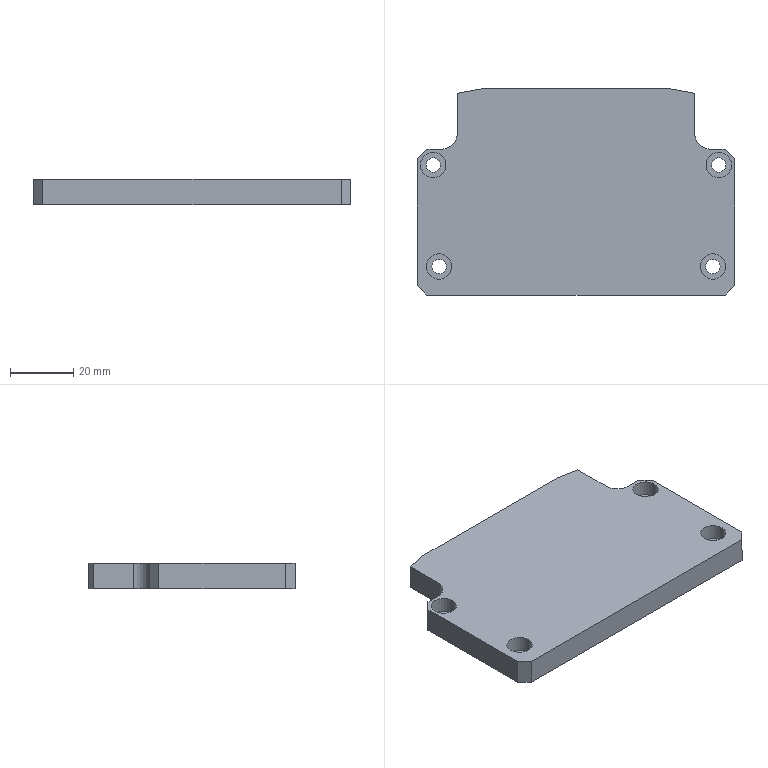Part | SolidWorks | features Chamfer 4, MoveFace 3, Fillet 2, HoleWzd 2, ICE 2, Extrusion 1 | 1 solid | 46 faces | box 100 x 65 x 8 mm | volume 46552 mm3 | cylinder 22 | plane 20 | cone 4 | commonest cylinder face diameters 4.5 x8 8 x8 3.3 x4 10 x2
STEP:
#1=CARTESIAN_POINT('',(-47.15,-14.,-1.));
#2=VERTEX_POINT('',#1);
#3=CARTESIAN_POINT('',(-39.15,-14.,-1.));
#4=VERTEX_POINT('',#3);
#5=CARTESIAN_POINT('',(-43.15,-14.,-1.));
#6=DIRECTION('',(0.,0.,1.));
#7=DIRECTION('',(1.,0.,0.));
#8=AXIS2_PLACEMENT_3D('',#5,#6,#7);
#9=CIRCLE('',#8,4.);
#10=EDGE_CURVE('',#2,#4,#9,.T.);
#11=ORIENTED_EDGE('',*,*,#10,.F.);
#12=CARTESIAN_POINT('',(-47.15,-14.,4.));
#13=VERTEX_POINT('',#12);
#14=CARTESIAN_POINT('',(-47.15,-14.,4.));
#15=DIRECTION('',(0.,0.,1.));
#16=VECTOR('',#15,1000.);
#17=LINE('',#14,#16);
#18=EDGE_CURVE('',#2,#13,#17,.T.);
#19=ORIENTED_EDGE('',*,*,#18,.T.);
#20=CARTESIAN_POINT('',(-39.15,-14.,4.));
#21=VERTEX_POINT('',#20);
#22=CARTESIAN_POINT('',(-43.15,-14.,4.));
#23=DIRECTION('',(0.,0.,1.));
#24=DIRECTION('',(1.,0.,0.));
#25=AXIS2_PLACEMENT_3D('',#22,#23,#24);
#26=CIRCLE('',#25,4.);
#27=EDGE_CURVE('',#13,#21,#26,.T.);
#28=ORIENTED_EDGE('',*,*,#27,.T.);
#29=CARTESIAN_POINT('',(-39.15,-14.,4.));
#30=DIRECTION('',(0.,0.,1.));
#31=VECTOR('',#30,1000.);
#32=LINE('',#29,#31);
#33=EDGE_CURVE('',#4,#21,#32,.T.);
#34=ORIENTED_EDGE('',*,*,#33,.F.);
#35=EDGE_LOOP('',(#11,#19,#28,#34));
#36=FACE_OUTER_BOUND('',#35,.T.);
#37=CARTESIAN_POINT('',(-43.15,-14.,4.));
#38=DIRECTION('',(0.,0.,1.));
#39=DIRECTION('',(1.,0.,0.));
#40=AXIS2_PLACEMENT_3D('',#37,#38,#39);
#41=CYLINDRICAL_SURFACE('',#40,4.);
#42=ADVANCED_FACE('',(#36),#41,.F.);
#43=CARTESIAN_POINT('',(-45.4,-14.,-4.));
#44=VERTEX_POINT('',#43);
#45=CARTESIAN_POINT('',(-40.9,-14.,-4.));
#46=VERTEX_POINT('',#45);
#47=CARTESIAN_POINT('',(-43.15,-14.,-4.));
#48=DIRECTION('',(0.,0.,1.));
#49=DIRECTION('',(1.,0.,0.));
#50=AXIS2_PLACEMENT_3D('',#47,#48,#49);
#51=CIRCLE('',#50,2.25);
#52=EDGE_CURVE('',#44,#46,#51,.T.);
#53=ORIENTED_EDGE('',*,*,#52,.F.);
#54=CARTESIAN_POINT('',(-45.4,-14.,-1.));
#55=VERTEX_POINT('',#54);
#56=CARTESIAN_POINT('',(-45.4,-14.,4.));
#57=DIRECTION('',(0.,0.,1.));
#58=VECTOR('',#57,1000.);
#59=LINE('',#56,#58);
#60=EDGE_CURVE('',#44,#55,#59,.T.);
#61=ORIENTED_EDGE('',*,*,#60,.T.);
#62=CARTESIAN_POINT('',(-40.9,-14.,-1.));
#63=VERTEX_POINT('',#62);
#64=CARTESIAN_POINT('',(-43.15,-14.,-1.));
#65=DIRECTION('',(0.,0.,1.));
#66=DIRECTION('',(1.,0.,0.));
#67=AXIS2_PLACEMENT_3D('',#64,#65,#66);
#68=CIRCLE('',#67,2.25);
#69=EDGE_CURVE('',#55,#63,#68,.T.);
#70=ORIENTED_EDGE('',*,*,#69,.T.);
#71=CARTESIAN_POINT('',(-40.9,-14.,4.));
#72=DIRECTION('',(0.,0.,1.));
#73=VECTOR('',#72,1000.);
#74=LINE('',#71,#73);
#75=EDGE_CURVE('',#46,#63,#74,.T.);
#76=ORIENTED_EDGE('',*,*,#75,.F.);
#77=EDGE_LOOP('',(#53,#61,#70,#76));
#78=FACE_OUTER_BOUND('',#77,.T.);
#79=CARTESIAN_POINT('',(-43.15,-14.,4.));
#80=DIRECTION('',(0.,0.,1.));
#81=DIRECTION('',(1.,0.,0.));
#82=AXIS2_PLACEMENT_3D('',#79,#80,#81);
#83=CYLINDRICAL_SURFACE('',#82,2.25);
#84=ADVANCED_FACE('',(#78),#83,.F.);
#85=CARTESIAN_POINT('',(39.15,-14.,-1.));
#86=VERTEX_POINT('',#85);
#87=CARTESIAN_POINT('',(47.15,-14.,-1.));
#88=VERTEX_POINT('',#87);
#89=CARTESIAN_POINT('',(43.15,-14.,-1.));
#90=DIRECTION('',(0.,0.,1.));
#91=DIRECTION('',(1.,0.,0.));
#92=AXIS2_PLACEMENT_3D('',#89,#90,#91);
#93=CIRCLE('',#92,4.);
#94=EDGE_CURVE('',#86,#88,#93,.T.);
#95=ORIENTED_EDGE('',*,*,#94,.F.);
#96=CARTESIAN_POINT('',(39.15,-14.,4.));
#97=VERTEX_POINT('',#96);
#98=CARTESIAN_POINT('',(39.15,-14.,4.));
#99=DIRECTION('',(0.,0.,1.));
#100=VECTOR('',#99,1000.);
#101=LINE('',#98,#100);
#102=EDGE_CURVE('',#86,#97,#101,.T.);
#103=ORIENTED_EDGE('',*,*,#102,.T.);
#104=CARTESIAN_POINT('',(47.15,-14.,4.));
#105=VERTEX_POINT('',#104);
#106=CARTESIAN_POINT('',(43.15,-14.,4.));
#107=DIRECTION('',(0.,0.,1.));
#108=DIRECTION('',(1.,0.,0.));
#109=AXIS2_PLACEMENT_3D('',#106,#107,#108);
#110=CIRCLE('',#109,4.);
#111=EDGE_CURVE('',#97,#105,#110,.T.);
#112=ORIENTED_EDGE('',*,*,#111,.T.);
#113=CARTESIAN_POINT('',(47.15,-14.,4.));
#114=DIRECTION('',(0.,0.,1.));
#115=VECTOR('',#114,1000.);
#116=LINE('',#113,#115);
#117=EDGE_CURVE('',#88,#105,#116,.T.);
#118=ORIENTED_EDGE('',*,*,#117,.F.);
#119=EDGE_LOOP('',(#95,#103,#112,#118));
#120=FACE_OUTER_BOUND('',#119,.T.);
#121=CARTESIAN_POINT('',(43.15,-14.,4.));
#122=DIRECTION('',(0.,0.,1.));
#123=DIRECTION('',(1.,0.,0.));
#124=AXIS2_PLACEMENT_3D('',#121,#122,#123);
#125=CYLINDRICAL_SURFACE('',#124,4.);
#126=ADVANCED_FACE('',(#120),#125,.F.);
#127=CARTESIAN_POINT('',(40.9,-14.,-4.));
#128=VERTEX_POINT('',#127);
#129=CARTESIAN_POINT('',(45.4,-14.,-4.));
#130=VERTEX_POINT('',#129);
#131=CARTESIAN_POINT('',(43.15,-14.,-4.));
#132=DIRECTION('',(0.,0.,1.));
#133=DIRECTION('',(1.,0.,0.));
#134=AXIS2_PLACEMENT_3D('',#131,#132,#133);
#135=CIRCLE('',#134,2.25);
#136=EDGE_CURVE('',#128,#130,#135,.T.);
#137=ORIENTED_EDGE('',*,*,#136,.F.);
#138=CARTESIAN_POINT('',(40.9,-14.,-1.));
#139=VERTEX_POINT('',#138);
#140=CARTESIAN_POINT('',(40.9,-14.,4.));
#141=DIRECTION('',(0.,0.,1.));
#142=VECTOR('',#141,1000.);
#143=LINE('',#140,#142);
#144=EDGE_CURVE('',#128,#139,#143,.T.);
#145=ORIENTED_EDGE('',*,*,#144,.T.);
#146=CARTESIAN_POINT('',(45.4,-14.,-1.));
#147=VERTEX_POINT('',#146);
#148=CARTESIAN_POINT('',(43.15,-14.,-1.));
#149=DIRECTION('',(0.,0.,1.));
#150=DIRECTION('',(1.,0.,0.));
#151=AXIS2_PLACEMENT_3D('',#148,#149,#150);
#152=CIRCLE('',#151,2.25);
#153=EDGE_CURVE('',#139,#147,#152,.T.);
#154=ORIENTED_EDGE('',*,*,#153,.T.);
#155=CARTESIAN_POINT('',(45.4,-14.,4.));
#156=DIRECTION('',(0.,0.,1.));
#157=VECTOR('',#156,1000.);
#158=LINE('',#155,#157);
#159=EDGE_CURVE('',#130,#147,#158,.T.);
#160=ORIENTED_EDGE('',*,*,#159,.F.);
#161=EDGE_LOOP('',(#137,#145,#154,#160));
#162=FACE_OUTER_BOUND('',#161,.T.);
#163=CARTESIAN_POINT('',(43.15,-14.,4.));
#164=DIRECTION('',(0.,0.,1.));
#165=DIRECTION('',(1.,0.,0.));
#166=AXIS2_PLACEMENT_3D('',#163,#164,#165);
#167=CYLINDRICAL_SURFACE('',#166,2.25);
#168=ADVANCED_FACE('',(#162),#167,.F.);
#169=CARTESIAN_POINT('',(-49.,18.,-1.));
#170=VERTEX_POINT('',#169);
#171=CARTESIAN_POINT('',(-41.,18.,-1.));
#172=VERTEX_POINT('',#171);
#173=CARTESIAN_POINT('',(-45.,18.,-1.));
#174=DIRECTION('',(0.,0.,1.));
#175=DIRECTION('',(1.,0.,0.));
#176=AXIS2_PLACEMENT_3D('',#173,#174,#175);
#177=CIRCLE('',#176,4.);
#178=EDGE_CURVE('',#170,#172,#177,.T.);
#179=ORIENTED_EDGE('',*,*,#178,.F.);
#180=CARTESIAN_POINT('',(-49.,18.,4.));
#181=VERTEX_POINT('',#180);
#182=CARTESIAN_POINT('',(-49.,18.,4.));
#183=DIRECTION('',(0.,0.,1.));
#184=VECTOR('',#183,1000.);
#185=LINE('',#182,#184);
#186=EDGE_CURVE('',#170,#181,#185,.T.);
#187=ORIENTED_EDGE('',*,*,#186,.T.);
#188=CARTESIAN_POINT('',(-41.,18.,4.));
#189=VERTEX_POINT('',#188);
#190=CARTESIAN_POINT('',(-45.,18.,4.));
#191=DIRECTION('',(0.,0.,1.));
#192=DIRECTION('',(1.,0.,0.));
#193=AXIS2_PLACEMENT_3D('',#190,#191,#192);
#194=CIRCLE('',#193,4.);
#195=EDGE_CURVE('',#181,#189,#194,.T.);
#196=ORIENTED_EDGE('',*,*,#195,.T.);
#197=CARTESIAN_POINT('',(-41.,18.,4.));
#198=DIRECTION('',(0.,0.,1.));
#199=VECTOR('',#198,1000.);
#200=LINE('',#197,#199);
#201=EDGE_CURVE('',#172,#189,#200,.T.);
#202=ORIENTED_EDGE('',*,*,#201,.F.);
#203=EDGE_LOOP('',(#179,#187,#196,#202));
#204=FACE_OUTER_BOUND('',#203,.T.);
#205=CARTESIAN_POINT('',(-45.,18.,4.));
#206=DIRECTION('',(0.,0.,1.));
#207=DIRECTION('',(1.,0.,0.));
#208=AXIS2_PLACEMENT_3D('',#205,#206,#207);
#209=CYLINDRICAL_SURFACE('',#208,4.);
#210=ADVANCED_FACE('',(#204),#209,.F.);
#211=CARTESIAN_POINT('',(-47.25,18.,-4.));
#212=VERTEX_POINT('',#211);
#213=CARTESIAN_POINT('',(-42.75,18.,-4.));
#214=VERTEX_POINT('',#213);
#215=CARTESIAN_POINT('',(-45.,18.,-4.));
#216=DIRECTION('',(0.,0.,1.));
#217=DIRECTION('',(1.,0.,0.));
#218=AXIS2_PLACEMENT_3D('',#215,#216,#217);
#219=CIRCLE('',#218,2.25);
#220=EDGE_CURVE('',#212,#214,#219,.T.);
#221=ORIENTED_EDGE('',*,*,#220,.F.);
#222=CARTESIAN_POINT('',(-47.25,18.,-1.));
#223=VERTEX_POINT('',#222);
#224=CARTESIAN_POINT('',(-47.25,18.,4.));
#225=DIRECTION('',(0.,0.,1.));
#226=VECTOR('',#225,1000.);
#227=LINE('',#224,#226);
#228=EDGE_CURVE('',#212,#223,#227,.T.);
#229=ORIENTED_EDGE('',*,*,#228,.T.);
#230=CARTESIAN_POINT('',(-42.75,18.,-1.));
#231=VERTEX_POINT('',#230);
#232=CARTESIAN_POINT('',(-45.,18.,-1.));
#233=DIRECTION('',(0.,0.,1.));
#234=DIRECTION('',(1.,0.,0.));
#235=AXIS2_PLACEMENT_3D('',#232,#233,#234);
#236=CIRCLE('',#235,2.25);
#237=EDGE_CURVE('',#223,#231,#236,.T.);
#238=ORIENTED_EDGE('',*,*,#237,.T.);
#239=CARTESIAN_POINT('',(-42.75,18.,4.));
#240=DIRECTION('',(0.,0.,1.));
#241=VECTOR('',#240,1000.);
#242=LINE('',#239,#241);
#243=EDGE_CURVE('',#214,#231,#242,.T.);
#244=ORIENTED_EDGE('',*,*,#243,.F.);
#245=EDGE_LOOP('',(#221,#229,#238,#244));
#246=FACE_OUTER_BOUND('',#245,.T.);
#247=CARTESIAN_POINT('',(-45.,18.,4.));
#248=DIRECTION('',(0.,0.,1.));
#249=DIRECTION('',(1.,0.,0.));
#250=AXIS2_PLACEMENT_3D('',#247,#248,#249);
#251=CYLINDRICAL_SURFACE('',#250,2.25);
#252=ADVANCED_FACE('',(#246),#251,.F.);
#253=CARTESIAN_POINT('',(41.,18.,-1.));
#254=VERTEX_POINT('',#253);
#255=CARTESIAN_POINT('',(49.,18.,-1.));
#256=VERTEX_POINT('',#255);
#257=CARTESIAN_POINT('',(45.,18.,-1.));
#258=DIRECTION('',(0.,0.,1.));
#259=DIRECTION('',(1.,0.,0.));
#260=AXIS2_PLACEMENT_3D('',#257,#258,#259);
#261=CIRCLE('',#260,4.);
#262=EDGE_CURVE('',#254,#256,#261,.T.);
#263=ORIENTED_EDGE('',*,*,#262,.F.);
#264=CARTESIAN_POINT('',(41.,18.,4.));
#265=VERTEX_POINT('',#264);
#266=CARTESIAN_POINT('',(41.,18.,4.));
#267=DIRECTION('',(0.,0.,1.));
#268=VECTOR('',#267,1000.);
#269=LINE('',#266,#268);
#270=EDGE_CURVE('',#254,#265,#269,.T.);
#271=ORIENTED_EDGE('',*,*,#270,.T.);
#272=CARTESIAN_POINT('',(49.,18.,4.));
#273=VERTEX_POINT('',#272);
#274=CARTESIAN_POINT('',(45.,18.,4.));
#275=DIRECTION('',(0.,0.,1.));
#276=DIRECTION('',(1.,0.,0.));
#277=AXIS2_PLACEMENT_3D('',#274,#275,#276);
#278=CIRCLE('',#277,4.);
#279=EDGE_CURVE('',#265,#273,#278,.T.);
#280=ORIENTED_EDGE('',*,*,#279,.T.);
#281=CARTESIAN_POINT('',(49.,18.,4.));
#282=DIRECTION('',(0.,0.,1.));
#283=VECTOR('',#282,1000.);
#284=LINE('',#281,#283);
#285=EDGE_CURVE('',#256,#273,#284,.T.);
#286=ORIENTED_EDGE('',*,*,#285,.F.);
#287=EDGE_LOOP('',(#263,#271,#280,#286));
#288=FACE_OUTER_BOUND('',#287,.T.);
#289=CARTESIAN_POINT('',(45.,18.,4.));
#290=DIRECTION('',(0.,0.,1.));
#291=DIRECTION('',(1.,0.,0.));
#292=AXIS2_PLACEMENT_3D('',#289,#290,#291);
#293=CYLINDRICAL_SURFACE('',#292,4.);
#294=ADVANCED_FACE('',(#288),#293,.F.);
#295=CARTESIAN_POINT('',(42.75,18.,-4.));
#296=VERTEX_POINT('',#295);
#297=CARTESIAN_POINT('',(47.25,18.,-4.));
#298=VERTEX_POINT('',#297);
#299=CARTESIAN_POINT('',(45.,18.,-4.));
#300=DIRECTION('',(0.,0.,1.));
#301=DIRECTION('',(1.,0.,0.));
#302=AXIS2_PLACEMENT_3D('',#299,#300,#301);
#303=CIRCLE('',#302,2.25);
#304=EDGE_CURVE('',#296,#298,#303,.T.);
#305=ORIENTED_EDGE('',*,*,#304,.F.);
#306=CARTESIAN_POINT('',(42.75,18.,-1.));
#307=VERTEX_POINT('',#306);
#308=CARTESIAN_POINT('',(42.75,18.,4.));
#309=DIRECTION('',(0.,0.,1.));
#310=VECTOR('',#309,1000.);
#311=LINE('',#308,#310);
#312=EDGE_CURVE('',#296,#307,#311,.T.);
#313=ORIENTED_EDGE('',*,*,#312,.T.);
#314=CARTESIAN_POINT('',(47.25,18.,-1.));
#315=VERTEX_POINT('',#314);
#316=CARTESIAN_POINT('',(45.,18.,-1.));
#317=DIRECTION('',(0.,0.,1.));
#318=DIRECTION('',(1.,0.,0.));
#319=AXIS2_PLACEMENT_3D('',#316,#317,#318);
#320=CIRCLE('',#319,2.25);
#321=EDGE_CURVE('',#307,#315,#320,.T.);
#322=ORIENTED_EDGE('',*,*,#321,.T.);
#323=CARTESIAN_POINT('',(47.25,18.,4.));
#324=DIRECTION('',(0.,0.,1.));
#325=VECTOR('',#324,1000.);
#326=LINE('',#323,#325);
#327=EDGE_CURVE('',#298,#315,#326,.T.);
#328=ORIENTED_EDGE('',*,*,#327,.F.);
#329=EDGE_LOOP('',(#305,#313,#322,#328));
#330=FACE_OUTER_BOUND('',#329,.T.);
#331=CARTESIAN_POINT('',(45.,18.,4.));
#332=DIRECTION('',(0.,0.,1.));
#333=DIRECTION('',(1.,0.,0.));
#334=AXIS2_PLACEMENT_3D('',#331,#332,#333);
#335=CYLINDRICAL_SURFACE('',#334,2.25);
#336=ADVANCED_FACE('',(#330),#335,.F.);
#337=CARTESIAN_POINT('',(20.,26.,-1.65));
#338=VERTEX_POINT('',#337);
#339=CARTESIAN_POINT('',(20.,26.,1.65));
#340=VERTEX_POINT('',#339);
#341=CARTESIAN_POINT('',(20.,26.,0.));
#342=DIRECTION('',(0.,1.,0.));
#343=DIRECTION('',(0.,0.,1.));
#344=AXIS2_PLACEMENT_3D('',#341,#342,#343);
#345=CIRCLE('',#344,1.65);
#346=EDGE_CURVE('',#338,#340,#345,.T.);
#347=ORIENTED_EDGE('',*,*,#346,.F.);
#348=CARTESIAN_POINT('',(20.,42.,-1.65));
#349=VERTEX_POINT('',#348);
#350=CARTESIAN_POINT('',(20.,38.,-1.65));
#351=DIRECTION('',(0.,1.,0.));
#352=VECTOR('',#351,1000.);
#353=LINE('',#350,#352);
#354=EDGE_CURVE('',#338,#349,#353,.T.);
#355=ORIENTED_EDGE('',*,*,#354,.T.);
#356=CARTESIAN_POINT('',(20.,42.,1.65));
#357=VERTEX_POINT('',#356);
#358=CARTESIAN_POINT('',(20.,42.,0.));
#359=DIRECTION('',(0.,1.,0.));
#360=DIRECTION('',(0.,0.,1.));
#361=AXIS2_PLACEMENT_3D('',#358,#359,#360);
#362=CIRCLE('',#361,1.65);
#363=EDGE_CURVE('',#349,#357,#362,.T.);
#364=ORIENTED_EDGE('',*,*,#363,.T.);
#365=CARTESIAN_POINT('',(20.,38.,1.65));
#366=DIRECTION('',(0.,1.,0.));
#367=VECTOR('',#366,1000.);
#368=LINE('',#365,#367);
#369=EDGE_CURVE('',#340,#357,#368,.T.);
#370=ORIENTED_EDGE('',*,*,#369,.F.);
#371=EDGE_LOOP('',(#347,#355,#364,#370));
#372=FACE_OUTER_BOUND('',#371,.T.);
#373=CARTESIAN_POINT('',(20.,38.,0.));
#374=DIRECTION('',(0.,1.,0.));
#375=DIRECTION('',(0.,0.,1.));
#376=AXIS2_PLACEMENT_3D('',#373,#374,#375);
#377=CYLINDRICAL_SURFACE('',#376,1.65);
#378=ADVANCED_FACE('',(#372),#377,.F.);
#379=CARTESIAN_POINT('',(20.,25.009,0.));
#380=VERTEX_POINT('',#379);
#381=CARTESIAN_POINT('',(20.,26.,1.65));
#382=DIRECTION('',(0.,0.515,0.8572));
#383=VECTOR('',#382,1000.);
#384=LINE('',#381,#383);
#385=EDGE_CURVE('',#380,#340,#384,.T.);
#386=ORIENTED_EDGE('',*,*,#385,.F.);
#387=CARTESIAN_POINT('',(20.,26.,-1.65));
#388=DIRECTION('',(0.,0.515,-0.8572));
#389=VECTOR('',#388,1000.);
#390=LINE('',#387,#389);
#391=EDGE_CURVE('',#380,#338,#390,.T.);
#392=ORIENTED_EDGE('',*,*,#391,.T.);
#393=ORIENTED_EDGE('',*,*,#346,.T.);
#394=EDGE_LOOP('',(#386,#392,#393));
#395=FACE_OUTER_BOUND('',#394,.T.);
#396=CARTESIAN_POINT('',(20.,26.,0.));
#397=DIRECTION('',(0.,1.,0.));
#398=DIRECTION('',(0.,0.,1.));
#399=AXIS2_PLACEMENT_3D('',#396,#397,#398);
#400=CONICAL_SURFACE('',#399,1.65,1.03);
#401=ADVANCED_FACE('',(#395),#400,.F.);
#402=CARTESIAN_POINT('',(-20.,26.,-1.65));
#403=VERTEX_POINT('',#402);
#404=CARTESIAN_POINT('',(-20.,26.,1.65));
#405=VERTEX_POINT('',#404);
#406=CARTESIAN_POINT('',(-20.,26.,0.));
#407=DIRECTION('',(0.,1.,0.));
#408=DIRECTION('',(0.,0.,1.));
#409=AXIS2_PLACEMENT_3D('',#406,#407,#408);
#410=CIRCLE('',#409,1.65);
#411=EDGE_CURVE('',#403,#405,#410,.T.);
#412=ORIENTED_EDGE('',*,*,#411,.F.);
#413=CARTESIAN_POINT('',(-20.,42.,-1.65));
#414=VERTEX_POINT('',#413);
#415=CARTESIAN_POINT('',(-20.,38.,-1.65));
#416=DIRECTION('',(0.,1.,0.));
#417=VECTOR('',#416,1000.);
#418=LINE('',#415,#417);
#419=EDGE_CURVE('',#403,#414,#418,.T.);
#420=ORIENTED_EDGE('',*,*,#419,.T.);
#421=CARTESIAN_POINT('',(-20.,42.,1.65));
#422=VERTEX_POINT('',#421);
#423=CARTESIAN_POINT('',(-20.,42.,0.));
#424=DIRECTION('',(0.,1.,0.));
#425=DIRECTION('',(0.,0.,1.));
#426=AXIS2_PLACEMENT_3D('',#423,#424,#425);
#427=CIRCLE('',#426,1.65);
#428=EDGE_CURVE('',#414,#422,#427,.T.);
#429=ORIENTED_EDGE('',*,*,#428,.T.);
#430=CARTESIAN_POINT('',(-20.,38.,1.65));
#431=DIRECTION('',(0.,1.,0.));
#432=VECTOR('',#431,1000.);
#433=LINE('',#430,#432);
#434=EDGE_CURVE('',#405,#422,#433,.T.);
#435=ORIENTED_EDGE('',*,*,#434,.F.);
#436=EDGE_LOOP('',(#412,#420,#429,#435));
#437=FACE_OUTER_BOUND('',#436,.T.);
#438=CARTESIAN_POINT('',(-20.,38.,0.));
#439=DIRECTION('',(0.,1.,0.));
#440=DIRECTION('',(0.,0.,1.));
#441=AXIS2_PLACEMENT_3D('',#438,#439,#440);
#442=CYLINDRICAL_SURFACE('',#441,1.65);
#443=ADVANCED_FACE('',(#437),#442,.F.);
#444=CARTESIAN_POINT('',(-20.,25.009,0.));
#445=VERTEX_POINT('',#444);
#446=CARTESIAN_POINT('',(-20.,26.,1.65));
#447=DIRECTION('',(0.,0.515,0.8572));
#448=VECTOR('',#447,1000.);
#449=LINE('',#446,#448);
#450=EDGE_CURVE('',#445,#405,#449,.T.);
#451=ORIENTED_EDGE('',*,*,#450,.F.);
#452=CARTESIAN_POINT('',(-20.,26.,-1.65));
#453=DIRECTION('',(0.,0.515,-0.8572));
#454=VECTOR('',#453,1000.);
#455=LINE('',#452,#454);
#456=EDGE_CURVE('',#445,#403,#455,.T.);
#457=ORIENTED_EDGE('',*,*,#456,.T.);
#458=ORIENTED_EDGE('',*,*,#411,.T.);
#459=EDGE_LOOP('',(#451,#457,#458));
#460=FACE_OUTER_BOUND('',#459,.T.);
#461=CARTESIAN_POINT('',(-20.,26.,0.));
#462=DIRECTION('',(0.,1.,0.));
#463=DIRECTION('',(0.,0.,1.));
#464=AXIS2_PLACEMENT_3D('',#461,#462,#463);
#465=CONICAL_SURFACE('',#464,1.65,1.03);
#466=ADVANCED_FACE('',(#460),#465,.F.);
#467=CARTESIAN_POINT('',(47.,23.,4.));
#468=VERTEX_POINT('',#467);
#469=CARTESIAN_POINT('',(42.4,23.,4.));
#470=VERTEX_POINT('',#469);
#471=CARTESIAN_POINT('',(-50.,23.,4.));
#472=DIRECTION('',(-1.,0.,0.));
#473=VECTOR('',#472,1000.);
#474=LINE('',#471,#473);
#475=EDGE_CURVE('',#468,#470,#474,.T.);
#476=ORIENTED_EDGE('',*,*,#475,.F.);
#477=CARTESIAN_POINT('',(47.,23.,-4.));
#478=VERTEX_POINT('',#477);
#479=CARTESIAN_POINT('',(47.,23.,4.));
#480=DIRECTION('',(0.,0.,-1.));
#481=VECTOR('',#480,1000.);
#482=LINE('',#479,#481);
#483=EDGE_CURVE('',#468,#478,#482,.T.);
#484=ORIENTED_EDGE('',*,*,#483,.T.);
#485=CARTESIAN_POINT('',(42.4,23.,-4.));
#486=VERTEX_POINT('',#485);
#487=CARTESIAN_POINT('',(-50.,23.,-4.));
#488=DIRECTION('',(-1.,0.,0.));
#489=VECTOR('',#488,1000.);
#490=LINE('',#487,#489);
#491=EDGE_CURVE('',#478,#486,#490,.T.);
#492=ORIENTED_EDGE('',*,*,#491,.T.);
#493=CARTESIAN_POINT('',(42.4,23.,4.));
#494=DIRECTION('',(0.,0.,1.));
#495=VECTOR('',#494,1000.);
#496=LINE('',#493,#495);
#497=EDGE_CURVE('',#486,#470,#496,.T.);
#498=ORIENTED_EDGE('',*,*,#497,.T.);
#499=EDGE_LOOP('',(#476,#484,#492,#498));
#500=FACE_OUTER_BOUND('',#499,.T.);
#501=CARTESIAN_POINT('',(-50.,23.,4.));
#502=DIRECTION('',(0.,-1.,0.));
#503=DIRECTION('',(0.,0.,-1.));
#504=AXIS2_PLACEMENT_3D('',#501,#502,#503);
#505=PLANE('',#504);
#506=ADVANCED_FACE('',(#500),#505,.F.);
#507=CARTESIAN_POINT('',(50.,-20.,-4.));
#508=VERTEX_POINT('',#507);
#509=CARTESIAN_POINT('',(50.,20.,-4.));
#510=VERTEX_POINT('',#509);
#511=CARTESIAN_POINT('',(50.,23.,-4.));
#512=DIRECTION('',(0.,1.,0.));
#513=VECTOR('',#512,1000.);
#514=LINE('',#511,#513);
#515=EDGE_CURVE('',#508,#510,#514,.T.);
#516=ORIENTED_EDGE('',*,*,#515,.T.);
#517=CARTESIAN_POINT('',(50.,20.,4.));
#518=VERTEX_POINT('',#517);
#519=CARTESIAN_POINT('',(50.,20.,4.));
#520=DIRECTION('',(0.,0.,1.));
#521=VECTOR('',#520,1000.);
#522=LINE('',#519,#521);
#523=EDGE_CURVE('',#510,#518,#522,.T.);
#524=ORIENTED_EDGE('',*,*,#523,.T.);
#525=CARTESIAN_POINT('',(50.,-20.,4.));
#526=VERTEX_POINT('',#525);
#527=CARTESIAN_POINT('',(50.,23.,4.));
#528=DIRECTION('',(0.,1.,0.));
#529=VECTOR('',#528,1000.);
#530=LINE('',#527,#529);
#531=EDGE_CURVE('',#526,#518,#530,.T.);
#532=ORIENTED_EDGE('',*,*,#531,.F.);
#533=CARTESIAN_POINT('',(50.,-20.,4.));
#534=DIRECTION('',(0.,0.,-1.));
#535=VECTOR('',#534,1000.);
#536=LINE('',#533,#535);
#537=EDGE_CURVE('',#526,#508,#536,.T.);
#538=ORIENTED_EDGE('',*,*,#537,.T.);
#539=EDGE_LOOP('',(#516,#524,#532,#538));
#540=FACE_OUTER_BOUND('',#539,.T.);
#541=CARTESIAN_POINT('',(50.,23.,4.));
#542=DIRECTION('',(-1.,0.,0.));
#543=DIRECTION('',(0.,0.,1.));
#544=AXIS2_PLACEMENT_3D('',#541,#542,#543);
#545=PLANE('',#544);
#546=ADVANCED_FACE('',(#540),#545,.F.);
#547=CARTESIAN_POINT('',(-42.4,23.,-4.));
#548=VERTEX_POINT('',#547);
#549=CARTESIAN_POINT('',(-47.,23.,-4.));
#550=VERTEX_POINT('',#549);
#551=CARTESIAN_POINT('',(-50.,23.,-4.));
#552=DIRECTION('',(-1.,0.,0.));
#553=VECTOR('',#552,1000.);
#554=LINE('',#551,#553);
#555=EDGE_CURVE('',#548,#550,#554,.T.);
#556=ORIENTED_EDGE('',*,*,#555,.T.);
#557=CARTESIAN_POINT('',(-47.,23.,4.));
#558=VERTEX_POINT('',#557);
#559=CARTESIAN_POINT('',(-47.,23.,4.));
#560=DIRECTION('',(0.,0.,1.));
#561=VECTOR('',#560,1000.);
#562=LINE('',#559,#561);
#563=EDGE_CURVE('',#550,#558,#562,.T.);
#564=ORIENTED_EDGE('',*,*,#563,.T.);
#565=CARTESIAN_POINT('',(-42.4,23.,4.));
#566=VERTEX_POINT('',#565);
#567=CARTESIAN_POINT('',(-50.,23.,4.));
#568=DIRECTION('',(-1.,0.,0.));
#569=VECTOR('',#568,1000.);
#570=LINE('',#567,#569);
#571=EDGE_CURVE('',#566,#558,#570,.T.);
#572=ORIENTED_EDGE('',*,*,#571,.F.);
#573=CARTESIAN_POINT('',(-42.4,23.,-4.));
#574=DIRECTION('',(0.,0.,-1.));
#575=VECTOR('',#574,1000.);
#576=LINE('',#573,#575);
#577=EDGE_CURVE('',#566,#548,#576,.T.);
#578=ORIENTED_EDGE('',*,*,#577,.T.);
#579=EDGE_LOOP('',(#556,#564,#572,#578));
#580=FACE_OUTER_BOUND('',#579,.T.);
#581=CARTESIAN_POINT('',(-50.,23.,4.));
#582=DIRECTION('',(0.,-1.,0.));
#583=DIRECTION('',(0.,0.,-1.));
#584=AXIS2_PLACEMENT_3D('',#581,#582,#583);
#585=PLANE('',#584);
#586=ADVANCED_FACE('',(#580),#585,.F.);
#587=CARTESIAN_POINT('',(-50.,20.,4.));
#588=VERTEX_POINT('',#587);
#589=CARTESIAN_POINT('',(-50.,-20.,4.));
#590=VERTEX_POINT('',#589);
#591=CARTESIAN_POINT('',(-50.,23.,4.));
#592=DIRECTION('',(0.,-1.,0.));
#593=VECTOR('',#592,1000.);
#594=LINE('',#591,#593);
#595=EDGE_CURVE('',#588,#590,#594,.T.);
#596=ORIENTED_EDGE('',*,*,#595,.F.);
#597=CARTESIAN_POINT('',(-50.,20.,-4.));
#598=VERTEX_POINT('',#597);
#599=CARTESIAN_POINT('',(-50.,20.,4.));
#600=DIRECTION('',(0.,0.,-1.));
#601=VECTOR('',#600,1000.);
#602=LINE('',#599,#601);
#603=EDGE_CURVE('',#588,#598,#602,.T.);
#604=ORIENTED_EDGE('',*,*,#603,.T.);
#605=CARTESIAN_POINT('',(-50.,-20.,-4.));
#606=VERTEX_POINT('',#605);
#607=CARTESIAN_POINT('',(-50.,23.,-4.));
#608=DIRECTION('',(0.,-1.,0.));
#609=VECTOR('',#608,1000.);
#610=LINE('',#607,#609);
#611=EDGE_CURVE('',#598,#606,#610,.T.);
#612=ORIENTED_EDGE('',*,*,#611,.T.);
#613=CARTESIAN_POINT('',(-50.,-20.,4.));
#614=DIRECTION('',(0.,0.,1.));
#615=VECTOR('',#614,1000.);
#616=LINE('',#613,#615);
#617=EDGE_CURVE('',#606,#590,#616,.T.);
#618=ORIENTED_EDGE('',*,*,#617,.T.);
#619=EDGE_LOOP('',(#596,#604,#612,#618));
#620=FACE_OUTER_BOUND('',#619,.T.);
#621=CARTESIAN_POINT('',(-50.,23.,4.));
#622=DIRECTION('',(1.,0.,0.));
#623=DIRECTION('',(0.,0.,-1.));
#624=AXIS2_PLACEMENT_3D('',#621,#622,#623);
#625=PLANE('',#624);
#626=ADVANCED_FACE('',(#620),#625,.F.);
#627=CARTESIAN_POINT('',(-47.,-23.,-4.));
#628=VERTEX_POINT('',#627);
#629=CARTESIAN_POINT('',(47.,-23.,-4.));
#630=VERTEX_POINT('',#629);
#631=CARTESIAN_POINT('',(-50.,-23.,-4.));
#632=DIRECTION('',(1.,0.,0.));
#633=VECTOR('',#632,1000.);
#634=LINE('',#631,#633);
#635=EDGE_CURVE('',#628,#630,#634,.T.);
#636=ORIENTED_EDGE('',*,*,#635,.T.);
#637=CARTESIAN_POINT('',(47.,-23.,4.));
#638=VERTEX_POINT('',#637);
#639=CARTESIAN_POINT('',(47.,-23.,4.));
#640=DIRECTION('',(0.,0.,1.));
#641=VECTOR('',#640,1000.);
#642=LINE('',#639,#641);
#643=EDGE_CURVE('',#630,#638,#642,.T.);
#644=ORIENTED_EDGE('',*,*,#643,.T.);
#645=CARTESIAN_POINT('',(-47.,-23.,4.));
#646=VERTEX_POINT('',#645);
#647=CARTESIAN_POINT('',(-50.,-23.,4.));
#648=DIRECTION('',(1.,0.,0.));
#649=VECTOR('',#648,1000.);
#650=LINE('',#647,#649);
#651=EDGE_CURVE('',#646,#638,#650,.T.);
#652=ORIENTED_EDGE('',*,*,#651,.F.);
#653=CARTESIAN_POINT('',(-47.,-23.,4.));
#654=DIRECTION('',(0.,0.,-1.));
#655=VECTOR('',#654,1000.);
#656=LINE('',#653,#655);
#657=EDGE_CURVE('',#646,#628,#656,.T.);
#658=ORIENTED_EDGE('',*,*,#657,.T.);
#659=EDGE_LOOP('',(#636,#644,#652,#658));
#660=FACE_OUTER_BOUND('',#659,.T.);
#661=CARTESIAN_POINT('',(-50.,-23.,4.));
#662=DIRECTION('',(0.,1.,0.));
#663=DIRECTION('',(0.,0.,1.));
#664=AXIS2_PLACEMENT_3D('',#661,#662,#663);
#665=PLANE('',#664);
#666=ADVANCED_FACE('',(#660),#665,.F.);
#667=CARTESIAN_POINT('',(-43.15,-14.,4.));
#668=DIRECTION('',(0.,0.,1.));
#669=DIRECTION('',(1.,0.,0.));
#670=AXIS2_PLACEMENT_3D('',#667,#668,#669);
#671=CIRCLE('',#670,4.);
#672=EDGE_CURVE('',#21,#13,#671,.T.);
#673=ORIENTED_EDGE('',*,*,#672,.F.);
#674=ORIENTED_EDGE('',*,*,#27,.F.);
#675=EDGE_LOOP('',(#673,#674));
#676=FACE_BOUND('',#675,.T.);
#677=CARTESIAN_POINT('',(43.15,-14.,4.));
#678=DIRECTION('',(0.,0.,1.));
#679=DIRECTION('',(1.,0.,0.));
#680=AXIS2_PLACEMENT_3D('',#677,#678,#679);
#681=CIRCLE('',#680,4.);
#682=EDGE_CURVE('',#105,#97,#681,.T.);
#683=ORIENTED_EDGE('',*,*,#682,.F.);
#684=ORIENTED_EDGE('',*,*,#111,.F.);
#685=EDGE_LOOP('',(#683,#684));
#686=FACE_BOUND('',#685,.T.);
#687=CARTESIAN_POINT('',(-45.,18.,4.));
#688=DIRECTION('',(0.,0.,1.));
#689=DIRECTION('',(1.,0.,0.));
#690=AXIS2_PLACEMENT_3D('',#687,#688,#689);
#691=CIRCLE('',#690,4.);
#692=EDGE_CURVE('',#189,#181,#691,.T.);
#693=ORIENTED_EDGE('',*,*,#692,.F.);
#694=ORIENTED_EDGE('',*,*,#195,.F.);
#695=EDGE_LOOP('',(#693,#694));
#696=FACE_BOUND('',#695,.T.);
#697=CARTESIAN_POINT('',(45.,18.,4.));
#698=DIRECTION('',(0.,0.,1.));
#699=DIRECTION('',(1.,0.,0.));
#700=AXIS2_PLACEMENT_3D('',#697,#698,#699);
#701=CIRCLE('',#700,4.);
#702=EDGE_CURVE('',#273,#265,#701,.T.);
#703=ORIENTED_EDGE('',*,*,#702,.F.);
#704=ORIENTED_EDGE('',*,*,#279,.F.);
#705=EDGE_LOOP('',(#703,#704));
#706=FACE_BOUND('',#705,.T.);
#707=ORIENTED_EDGE('',*,*,#571,.T.);
#708=CARTESIAN_POINT('',(-35.,35.,4.));
#709=DIRECTION('',(-0.7071,-0.7071,0.));
#710=VECTOR('',#709,1000.);
#711=LINE('',#708,#710);
#712=EDGE_CURVE('',#558,#588,#711,.T.);
#713=ORIENTED_EDGE('',*,*,#712,.T.);
#714=ORIENTED_EDGE('',*,*,#595,.T.);
#715=CARTESIAN_POINT('',(-35.,-35.,4.));
#716=DIRECTION('',(0.7071,-0.7071,0.));
#717=VECTOR('',#716,1000.);
#718=LINE('',#715,#717);
#719=EDGE_CURVE('',#590,#646,#718,.T.);
#720=ORIENTED_EDGE('',*,*,#719,.T.);
#721=ORIENTED_EDGE('',*,*,#651,.T.);
#722=CARTESIAN_POINT('',(35.,-35.,4.));
#723=DIRECTION('',(0.7071,0.7071,0.));
#724=VECTOR('',#723,1000.);
#725=LINE('',#722,#724);
#726=EDGE_CURVE('',#638,#526,#725,.T.);
#727=ORIENTED_EDGE('',*,*,#726,.T.);
#728=ORIENTED_EDGE('',*,*,#531,.T.);
#729=CARTESIAN_POINT('',(35.,35.,4.));
#730=DIRECTION('',(-0.7071,0.7071,0.));
#731=VECTOR('',#730,1000.);
#732=LINE('',#729,#731);
#733=EDGE_CURVE('',#518,#468,#732,.T.);
#734=ORIENTED_EDGE('',*,*,#733,.T.);
#735=ORIENTED_EDGE('',*,*,#475,.T.);
#736=CARTESIAN_POINT('',(37.4,28.,4.));
#737=VERTEX_POINT('',#736);
#738=CARTESIAN_POINT('',(42.4,28.,4.));
#739=DIRECTION('',(0.,0.,-1.));
#740=DIRECTION('',(1.,0.,0.));
#741=AXIS2_PLACEMENT_3D('',#738,#739,#740);
#742=CIRCLE('',#741,5.);
#743=EDGE_CURVE('',#470,#737,#742,.T.);
#744=ORIENTED_EDGE('',*,*,#743,.T.);
#745=CARTESIAN_POINT('',(37.4,40.618,4.));
#746=VERTEX_POINT('',#745);
#747=CARTESIAN_POINT('',(37.4,38.,4.));
#748=DIRECTION('',(0.,1.,0.));
#749=VECTOR('',#748,1000.);
#750=LINE('',#747,#749);
#751=EDGE_CURVE('',#737,#746,#750,.T.);
#752=ORIENTED_EDGE('',*,*,#751,.T.);
#753=CARTESIAN_POINT('',(29.8,42.,4.));
#754=VERTEX_POINT('',#753);
#755=CARTESIAN_POINT('',(7.642,46.029,4.));
#756=DIRECTION('',(-0.9839,0.1789,0.));
#757=VECTOR('',#756,1000.);
#758=LINE('',#755,#757);
#759=EDGE_CURVE('',#746,#754,#758,.T.);
#760=ORIENTED_EDGE('',*,*,#759,.T.);
#761=CARTESIAN_POINT('',(-29.8,42.,4.));
#762=VERTEX_POINT('',#761);
#763=CARTESIAN_POINT('',(-37.5,42.,4.));
#764=DIRECTION('',(-1.,0.,0.));
#765=VECTOR('',#764,1000.);
#766=LINE('',#763,#765);
#767=EDGE_CURVE('',#754,#762,#766,.T.);
#768=ORIENTED_EDGE('',*,*,#767,.T.);
#769=CARTESIAN_POINT('',(-37.4,40.618,4.));
#770=VERTEX_POINT('',#769);
#771=CARTESIAN_POINT('',(-7.642,46.029,4.));
#772=DIRECTION('',(-0.9839,-0.1789,0.));
#773=VECTOR('',#772,1000.);
#774=LINE('',#771,#773);
#775=EDGE_CURVE('',#762,#770,#774,.T.);
#776=ORIENTED_EDGE('',*,*,#775,.T.);
#777=CARTESIAN_POINT('',(-37.4,28.,4.));
#778=VERTEX_POINT('',#777);
#779=CARTESIAN_POINT('',(-37.4,38.,4.));
#780=DIRECTION('',(0.,-1.,0.));
#781=VECTOR('',#780,1000.);
#782=LINE('',#779,#781);
#783=EDGE_CURVE('',#770,#778,#782,.T.);
#784=ORIENTED_EDGE('',*,*,#783,.T.);
#785=CARTESIAN_POINT('',(-42.4,28.,4.));
#786=DIRECTION('',(0.,0.,-1.));
#787=DIRECTION('',(1.,0.,0.));
#788=AXIS2_PLACEMENT_3D('',#785,#786,#787);
#789=CIRCLE('',#788,5.);
#790=EDGE_CURVE('',#778,#566,#789,.T.);
#791=ORIENTED_EDGE('',*,*,#790,.T.);
#792=EDGE_LOOP('',(#707,#713,#714,#720,#721,#727,#728,#734,#735,#744,#752,#760,#768,#776,#784,#791));
#793=FACE_OUTER_BOUND('',#792,.T.);
#794=CARTESIAN_POINT('',(0.,0.,4.));
#795=DIRECTION('',(0.,0.,1.));
#796=DIRECTION('',(1.,0.,0.));
#797=AXIS2_PLACEMENT_3D('',#794,#795,#796);
#798=PLANE('',#797);
#799=ADVANCED_FACE('',(#676,#686,#696,#706,#793),#798,.T.);
#800=CARTESIAN_POINT('',(-43.15,-14.,-4.));
#801=DIRECTION('',(0.,0.,1.));
#802=DIRECTION('',(1.,0.,0.));
#803=AXIS2_PLACEMENT_3D('',#800,#801,#802);
#804=CIRCLE('',#803,2.25);
#805=EDGE_CURVE('',#46,#44,#804,.T.);
#806=ORIENTED_EDGE('',*,*,#805,.T.);
#807=ORIENTED_EDGE('',*,*,#52,.T.);
#808=EDGE_LOOP('',(#806,#807));
#809=FACE_BOUND('',#808,.T.);
#810=CARTESIAN_POINT('',(43.15,-14.,-4.));
#811=DIRECTION('',(0.,0.,1.));
#812=DIRECTION('',(1.,0.,0.));
#813=AXIS2_PLACEMENT_3D('',#810,#811,#812);
#814=CIRCLE('',#813,2.25);
#815=EDGE_CURVE('',#130,#128,#814,.T.);
#816=ORIENTED_EDGE('',*,*,#815,.T.);
#817=ORIENTED_EDGE('',*,*,#136,.T.);
#818=EDGE_LOOP('',(#816,#817));
#819=FACE_BOUND('',#818,.T.);
#820=CARTESIAN_POINT('',(-45.,18.,-4.));
#821=DIRECTION('',(0.,0.,1.));
#822=DIRECTION('',(1.,0.,0.));
#823=AXIS2_PLACEMENT_3D('',#820,#821,#822);
#824=CIRCLE('',#823,2.25);
#825=EDGE_CURVE('',#214,#212,#824,.T.);
#826=ORIENTED_EDGE('',*,*,#825,.T.);
#827=ORIENTED_EDGE('',*,*,#220,.T.);
#828=EDGE_LOOP('',(#826,#827));
#829=FACE_BOUND('',#828,.T.);
#830=CARTESIAN_POINT('',(45.,18.,-4.));
#831=DIRECTION('',(0.,0.,1.));
#832=DIRECTION('',(1.,0.,0.));
#833=AXIS2_PLACEMENT_3D('',#830,#831,#832);
#834=CIRCLE('',#833,2.25);
#835=EDGE_CURVE('',#298,#296,#834,.T.);
#836=ORIENTED_EDGE('',*,*,#835,.T.);
#837=ORIENTED_EDGE('',*,*,#304,.T.);
#838=EDGE_LOOP('',(#836,#837));
#839=FACE_BOUND('',#838,.T.);
#840=ORIENTED_EDGE('',*,*,#611,.F.);
#841=CARTESIAN_POINT('',(-50.,20.,-4.));
#842=DIRECTION('',(0.7071,0.7071,0.));
#843=VECTOR('',#842,1000.);
#844=LINE('',#841,#843);
#845=EDGE_CURVE('',#598,#550,#844,.T.);
#846=ORIENTED_EDGE('',*,*,#845,.T.);
#847=ORIENTED_EDGE('',*,*,#555,.F.);
#848=CARTESIAN_POINT('',(-37.4,28.,-4.));
#849=VERTEX_POINT('',#848);
#850=CARTESIAN_POINT('',(-42.4,28.,-4.));
#851=DIRECTION('',(0.,0.,1.));
#852=DIRECTION('',(1.,0.,0.));
#853=AXIS2_PLACEMENT_3D('',#850,#851,#852);
#854=CIRCLE('',#853,5.);
#855=EDGE_CURVE('',#548,#849,#854,.T.);
#856=ORIENTED_EDGE('',*,*,#855,.T.);
#857=CARTESIAN_POINT('',(-37.4,40.618,-4.));
#858=VERTEX_POINT('',#857);
#859=CARTESIAN_POINT('',(-37.4,38.,-4.));
#860=DIRECTION('',(0.,-1.,0.));
#861=VECTOR('',#860,1000.);
#862=LINE('',#859,#861);
#863=EDGE_CURVE('',#858,#849,#862,.T.);
#864=ORIENTED_EDGE('',*,*,#863,.F.);
#865=CARTESIAN_POINT('',(-29.8,42.,-4.));
#866=VERTEX_POINT('',#865);
#867=CARTESIAN_POINT('',(-37.5,40.6,-4.));
#868=DIRECTION('',(0.9839,0.1789,0.));
#869=VECTOR('',#868,1000.);
#870=LINE('',#867,#869);
#871=EDGE_CURVE('',#858,#866,#870,.T.);
#872=ORIENTED_EDGE('',*,*,#871,.T.);
#873=CARTESIAN_POINT('',(29.8,42.,-4.));
#874=VERTEX_POINT('',#873);
#875=CARTESIAN_POINT('',(-37.5,42.,-4.));
#876=DIRECTION('',(-1.,0.,0.));
#877=VECTOR('',#876,1000.);
#878=LINE('',#875,#877);
#879=EDGE_CURVE('',#874,#866,#878,.T.);
#880=ORIENTED_EDGE('',*,*,#879,.F.);
#881=CARTESIAN_POINT('',(37.4,40.618,-4.));
#882=VERTEX_POINT('',#881);
#883=CARTESIAN_POINT('',(29.8,42.,-4.));
#884=DIRECTION('',(0.9839,-0.1789,0.));
#885=VECTOR('',#884,1000.);
#886=LINE('',#883,#885);
#887=EDGE_CURVE('',#874,#882,#886,.T.);
#888=ORIENTED_EDGE('',*,*,#887,.T.);
#889=CARTESIAN_POINT('',(37.4,28.,-4.));
#890=VERTEX_POINT('',#889);
#891=CARTESIAN_POINT('',(37.4,38.,-4.));
#892=DIRECTION('',(0.,1.,0.));
#893=VECTOR('',#892,1000.);
#894=LINE('',#891,#893);
#895=EDGE_CURVE('',#890,#882,#894,.T.);
#896=ORIENTED_EDGE('',*,*,#895,.F.);
#897=CARTESIAN_POINT('',(42.4,28.,-4.));
#898=DIRECTION('',(0.,0.,1.));
#899=DIRECTION('',(1.,0.,0.));
#900=AXIS2_PLACEMENT_3D('',#897,#898,#899);
#901=CIRCLE('',#900,5.);
#902=EDGE_CURVE('',#890,#486,#901,.T.);
#903=ORIENTED_EDGE('',*,*,#902,.T.);
#904=ORIENTED_EDGE('',*,*,#491,.F.);
#905=CARTESIAN_POINT('',(47.,23.,-4.));
#906=DIRECTION('',(0.7071,-0.7071,0.));
#907=VECTOR('',#906,1000.);
#908=LINE('',#905,#907);
#909=EDGE_CURVE('',#478,#510,#908,.T.);
#910=ORIENTED_EDGE('',*,*,#909,.T.);
#911=ORIENTED_EDGE('',*,*,#515,.F.);
#912=CARTESIAN_POINT('',(50.,-20.,-4.));
#913=DIRECTION('',(-0.7071,-0.7071,0.));
#914=VECTOR('',#913,1000.);
#915=LINE('',#912,#914);
#916=EDGE_CURVE('',#508,#630,#915,.T.);
#917=ORIENTED_EDGE('',*,*,#916,.T.);
#918=ORIENTED_EDGE('',*,*,#635,.F.);
#919=CARTESIAN_POINT('',(-47.,-23.,-4.));
#920=DIRECTION('',(-0.7071,0.7071,0.));
#921=VECTOR('',#920,1000.);
#922=LINE('',#919,#921);
#923=EDGE_CURVE('',#628,#606,#922,.T.);
#924=ORIENTED_EDGE('',*,*,#923,.T.);
#925=EDGE_LOOP('',(#840,#846,#847,#856,#864,#872,#880,#888,#896,#903,#904,#910,#911,#917,#918,#924));
#926=FACE_OUTER_BOUND('',#925,.T.);
#927=CARTESIAN_POINT('',(0.,0.,-4.));
#928=DIRECTION('',(0.,0.,1.));
#929=DIRECTION('',(1.,0.,0.));
#930=AXIS2_PLACEMENT_3D('',#927,#928,#929);
#931=PLANE('',#930);
#932=ADVANCED_FACE('',(#809,#819,#829,#839,#926),#931,.F.);
#933=ORIENTED_EDGE('',*,*,#751,.F.);
#934=CARTESIAN_POINT('',(37.4,28.,-4.));
#935=DIRECTION('',(0.,0.,-1.));
#936=VECTOR('',#935,1000.);
#937=LINE('',#934,#936);
#938=EDGE_CURVE('',#737,#890,#937,.T.);
#939=ORIENTED_EDGE('',*,*,#938,.T.);
#940=ORIENTED_EDGE('',*,*,#895,.T.);
#941=CARTESIAN_POINT('',(37.4,40.618,4.));
#942=DIRECTION('',(0.,0.,1.));
#943=VECTOR('',#942,1000.);
#944=LINE('',#941,#943);
#945=EDGE_CURVE('',#882,#746,#944,.T.);
#946=ORIENTED_EDGE('',*,*,#945,.T.);
#947=EDGE_LOOP('',(#933,#939,#940,#946));
#948=FACE_OUTER_BOUND('',#947,.T.);
#949=CARTESIAN_POINT('',(37.4,38.,4.));
#950=DIRECTION('',(-1.,0.,0.));
#951=DIRECTION('',(0.,0.,1.));
#952=AXIS2_PLACEMENT_3D('',#949,#950,#951);
#953=PLANE('',#952);
#954=ADVANCED_FACE('',(#948),#953,.F.);
#955=CARTESIAN_POINT('',(20.,42.,0.));
#956=DIRECTION('',(0.,1.,0.));
#957=DIRECTION('',(0.,0.,1.));
#958=AXIS2_PLACEMENT_3D('',#955,#956,#957);
#959=CIRCLE('',#958,1.65);
#960=EDGE_CURVE('',#357,#349,#959,.T.);
#961=ORIENTED_EDGE('',*,*,#960,.F.);
#962=ORIENTED_EDGE('',*,*,#363,.F.);
#963=EDGE_LOOP('',(#961,#962));
#964=FACE_BOUND('',#963,.T.);
#965=CARTESIAN_POINT('',(-20.,42.,0.));
#966=DIRECTION('',(0.,1.,0.));
#967=DIRECTION('',(0.,0.,1.));
#968=AXIS2_PLACEMENT_3D('',#965,#966,#967);
#969=CIRCLE('',#968,1.65);
#970=EDGE_CURVE('',#422,#414,#969,.T.);
#971=ORIENTED_EDGE('',*,*,#970,.F.);
#972=ORIENTED_EDGE('',*,*,#428,.F.);
#973=EDGE_LOOP('',(#971,#972));
#974=FACE_BOUND('',#973,.T.);
#975=ORIENTED_EDGE('',*,*,#767,.F.);
#976=CARTESIAN_POINT('',(29.8,42.,4.));
#977=DIRECTION('',(0.,0.,-1.));
#978=VECTOR('',#977,1000.);
#979=LINE('',#976,#978);
#980=EDGE_CURVE('',#754,#874,#979,.T.);
#981=ORIENTED_EDGE('',*,*,#980,.T.);
#982=ORIENTED_EDGE('',*,*,#879,.T.);
#983=CARTESIAN_POINT('',(-29.8,42.,4.));
#984=DIRECTION('',(0.,0.,1.));
#985=VECTOR('',#984,1000.);
#986=LINE('',#983,#985);
#987=EDGE_CURVE('',#866,#762,#986,.T.);
#988=ORIENTED_EDGE('',*,*,#987,.T.);
#989=EDGE_LOOP('',(#975,#981,#982,#988));
#990=FACE_OUTER_BOUND('',#989,.T.);
#991=CARTESIAN_POINT('',(-37.5,42.,4.));
#992=DIRECTION('',(0.,-1.,0.));
#993=DIRECTION('',(0.,0.,-1.));
#994=AXIS2_PLACEMENT_3D('',#991,#992,#993);
#995=PLANE('',#994);
#996=ADVANCED_FACE('',(#964,#974,#990),#995,.F.);
#997=ORIENTED_EDGE('',*,*,#863,.T.);
#998=CARTESIAN_POINT('',(-37.4,28.,4.));
#999=DIRECTION('',(0.,0.,1.));
#1000=VECTOR('',#999,1000.);
#1001=LINE('',#998,#1000);
#1002=EDGE_CURVE('',#849,#778,#1001,.T.);
#1003=ORIENTED_EDGE('',*,*,#1002,.T.);
#1004=ORIENTED_EDGE('',*,*,#783,.F.);
#1005=CARTESIAN_POINT('',(-37.4,40.618,4.));
#1006=DIRECTION('',(0.,0.,-1.));
#1007=VECTOR('',#1006,1000.);
#1008=LINE('',#1005,#1007);
#1009=EDGE_CURVE('',#770,#858,#1008,.T.);
#1010=ORIENTED_EDGE('',*,*,#1009,.T.);
#1011=EDGE_LOOP('',(#997,#1003,#1004,#1010));
#1012=FACE_OUTER_BOUND('',#1011,.T.);
#1013=CARTESIAN_POINT('',(-37.4,38.,4.));
#1014=DIRECTION('',(1.,0.,0.));
#1015=DIRECTION('',(0.,0.,-1.));
#1016=AXIS2_PLACEMENT_3D('',#1013,#1014,#1015);
#1017=PLANE('',#1016);
#1018=ADVANCED_FACE('',(#1012),#1017,.F.);
#1019=ORIENTED_EDGE('',*,*,#775,.F.);
#1020=ORIENTED_EDGE('',*,*,#987,.F.);
#1021=ORIENTED_EDGE('',*,*,#871,.F.);
#1022=ORIENTED_EDGE('',*,*,#1009,.F.);
#1023=EDGE_LOOP('',(#1019,#1020,#1021,#1022));
#1024=FACE_OUTER_BOUND('',#1023,.T.);
#1025=CARTESIAN_POINT('',(-37.5,40.6,4.));
#1026=DIRECTION('',(0.1789,-0.9839,0.));
#1027=DIRECTION('',(0.,0.,-1.));
#1028=AXIS2_PLACEMENT_3D('',#1025,#1026,#1027);
#1029=PLANE('',#1028);
#1030=ADVANCED_FACE('',(#1024),#1029,.F.);
#1031=ORIENTED_EDGE('',*,*,#759,.F.);
#1032=ORIENTED_EDGE('',*,*,#945,.F.);
#1033=ORIENTED_EDGE('',*,*,#887,.F.);
#1034=ORIENTED_EDGE('',*,*,#980,.F.);
#1035=EDGE_LOOP('',(#1031,#1032,#1033,#1034));
#1036=FACE_OUTER_BOUND('',#1035,.T.);
#1037=CARTESIAN_POINT('',(29.8,42.,4.));
#1038=DIRECTION('',(-0.1789,-0.9839,0.));
#1039=DIRECTION('',(0.,0.,-1.));
#1040=AXIS2_PLACEMENT_3D('',#1037,#1038,#1039);
#1041=PLANE('',#1040);
#1042=ADVANCED_FACE('',(#1036),#1041,.F.);
#1043=ORIENTED_EDGE('',*,*,#790,.F.);
#1044=ORIENTED_EDGE('',*,*,#1002,.F.);
#1045=ORIENTED_EDGE('',*,*,#855,.F.);
#1046=ORIENTED_EDGE('',*,*,#577,.F.);
#1047=EDGE_LOOP('',(#1043,#1044,#1045,#1046));
#1048=FACE_OUTER_BOUND('',#1047,.T.);
#1049=CARTESIAN_POINT('',(-42.4,28.,4.));
#1050=DIRECTION('',(0.,0.,1.));
#1051=DIRECTION('',(1.,0.,0.));
#1052=AXIS2_PLACEMENT_3D('',#1049,#1050,#1051);
#1053=CYLINDRICAL_SURFACE('',#1052,5.);
#1054=ADVANCED_FACE('',(#1048),#1053,.F.);
#1055=ORIENTED_EDGE('',*,*,#743,.F.);
#1056=ORIENTED_EDGE('',*,*,#497,.F.);
#1057=ORIENTED_EDGE('',*,*,#902,.F.);
#1058=ORIENTED_EDGE('',*,*,#938,.F.);
#1059=EDGE_LOOP('',(#1055,#1056,#1057,#1058));
#1060=FACE_OUTER_BOUND('',#1059,.T.);
#1061=CARTESIAN_POINT('',(42.4,28.,4.));
#1062=DIRECTION('',(0.,0.,1.));
#1063=DIRECTION('',(1.,0.,0.));
#1064=AXIS2_PLACEMENT_3D('',#1061,#1062,#1063);
#1065=CYLINDRICAL_SURFACE('',#1064,5.);
#1066=ADVANCED_FACE('',(#1060),#1065,.F.);
#1067=ORIENTED_EDGE('',*,*,#456,.F.);
#1068=ORIENTED_EDGE('',*,*,#450,.T.);
#1069=CARTESIAN_POINT('',(-20.,26.,0.));
#1070=DIRECTION('',(0.,1.,0.));
#1071=DIRECTION('',(0.,0.,1.));
#1072=AXIS2_PLACEMENT_3D('',#1069,#1070,#1071);
#1073=CIRCLE('',#1072,1.65);
#1074=EDGE_CURVE('',#405,#403,#1073,.T.);
#1075=ORIENTED_EDGE('',*,*,#1074,.T.);
#1076=EDGE_LOOP('',(#1067,#1068,#1075));
#1077=FACE_OUTER_BOUND('',#1076,.T.);
#1078=CARTESIAN_POINT('',(-20.,26.,0.));
#1079=DIRECTION('',(0.,1.,0.));
#1080=DIRECTION('',(0.,0.,1.));
#1081=AXIS2_PLACEMENT_3D('',#1078,#1079,#1080);
#1082=CONICAL_SURFACE('',#1081,1.65,1.03);
#1083=ADVANCED_FACE('',(#1077),#1082,.F.);
#1084=ORIENTED_EDGE('',*,*,#419,.F.);
#1085=ORIENTED_EDGE('',*,*,#1074,.F.);
#1086=ORIENTED_EDGE('',*,*,#434,.T.);
#1087=ORIENTED_EDGE('',*,*,#970,.T.);
#1088=EDGE_LOOP('',(#1084,#1085,#1086,#1087));
#1089=FACE_OUTER_BOUND('',#1088,.T.);
#1090=CARTESIAN_POINT('',(-20.,38.,0.));
#1091=DIRECTION('',(0.,1.,0.));
#1092=DIRECTION('',(0.,0.,1.));
#1093=AXIS2_PLACEMENT_3D('',#1090,#1091,#1092);
#1094=CYLINDRICAL_SURFACE('',#1093,1.65);
#1095=ADVANCED_FACE('',(#1089),#1094,.F.);
#1096=ORIENTED_EDGE('',*,*,#391,.F.);
#1097=ORIENTED_EDGE('',*,*,#385,.T.);
#1098=CARTESIAN_POINT('',(20.,26.,0.));
#1099=DIRECTION('',(0.,1.,0.));
#1100=DIRECTION('',(0.,0.,1.));
#1101=AXIS2_PLACEMENT_3D('',#1098,#1099,#1100);
#1102=CIRCLE('',#1101,1.65);
#1103=EDGE_CURVE('',#340,#338,#1102,.T.);
#1104=ORIENTED_EDGE('',*,*,#1103,.T.);
#1105=EDGE_LOOP('',(#1096,#1097,#1104));
#1106=FACE_OUTER_BOUND('',#1105,.T.);
#1107=CARTESIAN_POINT('',(20.,26.,0.));
#1108=DIRECTION('',(0.,1.,0.));
#1109=DIRECTION('',(0.,0.,1.));
#1110=AXIS2_PLACEMENT_3D('',#1107,#1108,#1109);
#1111=CONICAL_SURFACE('',#1110,1.65,1.03);
#1112=ADVANCED_FACE('',(#1106),#1111,.F.);
#1113=ORIENTED_EDGE('',*,*,#354,.F.);
#1114=ORIENTED_EDGE('',*,*,#1103,.F.);
#1115=ORIENTED_EDGE('',*,*,#369,.T.);
#1116=ORIENTED_EDGE('',*,*,#960,.T.);
#1117=EDGE_LOOP('',(#1113,#1114,#1115,#1116));
#1118=FACE_OUTER_BOUND('',#1117,.T.);
#1119=CARTESIAN_POINT('',(20.,38.,0.));
#1120=DIRECTION('',(0.,1.,0.));
#1121=DIRECTION('',(0.,0.,1.));
#1122=AXIS2_PLACEMENT_3D('',#1119,#1120,#1121);
#1123=CYLINDRICAL_SURFACE('',#1122,1.65);
#1124=ADVANCED_FACE('',(#1118),#1123,.F.);
#1125=ORIENTED_EDGE('',*,*,#312,.F.);
#1126=ORIENTED_EDGE('',*,*,#835,.F.);
#1127=ORIENTED_EDGE('',*,*,#327,.T.);
#1128=CARTESIAN_POINT('',(45.,18.,-1.));
#1129=DIRECTION('',(0.,0.,1.));
#1130=DIRECTION('',(1.,0.,0.));
#1131=AXIS2_PLACEMENT_3D('',#1128,#1129,#1130);
#1132=CIRCLE('',#1131,2.25);
#1133=EDGE_CURVE('',#315,#307,#1132,.T.);
#1134=ORIENTED_EDGE('',*,*,#1133,.T.);
#1135=EDGE_LOOP('',(#1125,#1126,#1127,#1134));
#1136=FACE_OUTER_BOUND('',#1135,.T.);
#1137=CARTESIAN_POINT('',(45.,18.,4.));
#1138=DIRECTION('',(0.,0.,1.));
#1139=DIRECTION('',(1.,0.,0.));
#1140=AXIS2_PLACEMENT_3D('',#1137,#1138,#1139);
#1141=CYLINDRICAL_SURFACE('',#1140,2.25);
#1142=ADVANCED_FACE('',(#1136),#1141,.F.);
#1143=ORIENTED_EDGE('',*,*,#1133,.F.);
#1144=ORIENTED_EDGE('',*,*,#321,.F.);
#1145=EDGE_LOOP('',(#1143,#1144));
#1146=FACE_BOUND('',#1145,.T.);
#1147=CARTESIAN_POINT('',(45.,18.,-1.));
#1148=DIRECTION('',(0.,0.,1.));
#1149=DIRECTION('',(1.,0.,0.));
#1150=AXIS2_PLACEMENT_3D('',#1147,#1148,#1149);
#1151=CIRCLE('',#1150,4.);
#1152=EDGE_CURVE('',#256,#254,#1151,.T.);
#1153=ORIENTED_EDGE('',*,*,#1152,.T.);
#1154=ORIENTED_EDGE('',*,*,#262,.T.);
#1155=EDGE_LOOP('',(#1153,#1154));
#1156=FACE_OUTER_BOUND('',#1155,.T.);
#1157=CARTESIAN_POINT('',(47.25,18.,-1.));
#1158=DIRECTION('',(0.,0.,-1.));
#1159=DIRECTION('',(-1.,0.,0.));
#1160=AXIS2_PLACEMENT_3D('',#1157,#1158,#1159);
#1161=PLANE('',#1160);
#1162=ADVANCED_FACE('',(#1146,#1156),#1161,.F.);
#1163=ORIENTED_EDGE('',*,*,#270,.F.);
#1164=ORIENTED_EDGE('',*,*,#1152,.F.);
#1165=ORIENTED_EDGE('',*,*,#285,.T.);
#1166=ORIENTED_EDGE('',*,*,#702,.T.);
#1167=EDGE_LOOP('',(#1163,#1164,#1165,#1166));
#1168=FACE_OUTER_BOUND('',#1167,.T.);
#1169=CARTESIAN_POINT('',(45.,18.,4.));
#1170=DIRECTION('',(0.,0.,1.));
#1171=DIRECTION('',(1.,0.,0.));
#1172=AXIS2_PLACEMENT_3D('',#1169,#1170,#1171);
#1173=CYLINDRICAL_SURFACE('',#1172,4.);
#1174=ADVANCED_FACE('',(#1168),#1173,.F.);
#1175=ORIENTED_EDGE('',*,*,#228,.F.);
#1176=ORIENTED_EDGE('',*,*,#825,.F.);
#1177=ORIENTED_EDGE('',*,*,#243,.T.);
#1178=CARTESIAN_POINT('',(-45.,18.,-1.));
#1179=DIRECTION('',(0.,0.,1.));
#1180=DIRECTION('',(1.,0.,0.));
#1181=AXIS2_PLACEMENT_3D('',#1178,#1179,#1180);
#1182=CIRCLE('',#1181,2.25);
#1183=EDGE_CURVE('',#231,#223,#1182,.T.);
#1184=ORIENTED_EDGE('',*,*,#1183,.T.);
#1185=EDGE_LOOP('',(#1175,#1176,#1177,#1184));
#1186=FACE_OUTER_BOUND('',#1185,.T.);
#1187=CARTESIAN_POINT('',(-45.,18.,4.));
#1188=DIRECTION('',(0.,0.,1.));
#1189=DIRECTION('',(1.,0.,0.));
#1190=AXIS2_PLACEMENT_3D('',#1187,#1188,#1189);
#1191=CYLINDRICAL_SURFACE('',#1190,2.25);
#1192=ADVANCED_FACE('',(#1186),#1191,.F.);
#1193=ORIENTED_EDGE('',*,*,#1183,.F.);
#1194=ORIENTED_EDGE('',*,*,#237,.F.);
#1195=EDGE_LOOP('',(#1193,#1194));
#1196=FACE_BOUND('',#1195,.T.);
#1197=CARTESIAN_POINT('',(-45.,18.,-1.));
#1198=DIRECTION('',(0.,0.,1.));
#1199=DIRECTION('',(1.,0.,0.));
#1200=AXIS2_PLACEMENT_3D('',#1197,#1198,#1199);
#1201=CIRCLE('',#1200,4.);
#1202=EDGE_CURVE('',#172,#170,#1201,.T.);
#1203=ORIENTED_EDGE('',*,*,#1202,.T.);
#1204=ORIENTED_EDGE('',*,*,#178,.T.);
#1205=EDGE_LOOP('',(#1203,#1204));
#1206=FACE_OUTER_BOUND('',#1205,.T.);
#1207=CARTESIAN_POINT('',(-42.75,18.,-1.));
#1208=DIRECTION('',(0.,0.,-1.));
#1209=DIRECTION('',(-1.,0.,0.));
#1210=AXIS2_PLACEMENT_3D('',#1207,#1208,#1209);
#1211=PLANE('',#1210);
#1212=ADVANCED_FACE('',(#1196,#1206),#1211,.F.);
#1213=ORIENTED_EDGE('',*,*,#186,.F.);
#1214=ORIENTED_EDGE('',*,*,#1202,.F.);
#1215=ORIENTED_EDGE('',*,*,#201,.T.);
#1216=ORIENTED_EDGE('',*,*,#692,.T.);
#1217=EDGE_LOOP('',(#1213,#1214,#1215,#1216));
#1218=FACE_OUTER_BOUND('',#1217,.T.);
#1219=CARTESIAN_POINT('',(-45.,18.,4.));
#1220=DIRECTION('',(0.,0.,1.));
#1221=DIRECTION('',(1.,0.,0.));
#1222=AXIS2_PLACEMENT_3D('',#1219,#1220,#1221);
#1223=CYLINDRICAL_SURFACE('',#1222,4.);
#1224=ADVANCED_FACE('',(#1218),#1223,.F.);
#1225=ORIENTED_EDGE('',*,*,#144,.F.);
#1226=ORIENTED_EDGE('',*,*,#815,.F.);
#1227=ORIENTED_EDGE('',*,*,#159,.T.);
#1228=CARTESIAN_POINT('',(43.15,-14.,-1.));
#1229=DIRECTION('',(0.,0.,1.));
#1230=DIRECTION('',(1.,0.,0.));
#1231=AXIS2_PLACEMENT_3D('',#1228,#1229,#1230);
#1232=CIRCLE('',#1231,2.25);
#1233=EDGE_CURVE('',#147,#139,#1232,.T.);
#1234=ORIENTED_EDGE('',*,*,#1233,.T.);
#1235=EDGE_LOOP('',(#1225,#1226,#1227,#1234));
#1236=FACE_OUTER_BOUND('',#1235,.T.);
#1237=CARTESIAN_POINT('',(43.15,-14.,4.));
#1238=DIRECTION('',(0.,0.,1.));
#1239=DIRECTION('',(1.,0.,0.));
#1240=AXIS2_PLACEMENT_3D('',#1237,#1238,#1239);
#1241=CYLINDRICAL_SURFACE('',#1240,2.25);
#1242=ADVANCED_FACE('',(#1236),#1241,.F.);
#1243=ORIENTED_EDGE('',*,*,#1233,.F.);
#1244=ORIENTED_EDGE('',*,*,#153,.F.);
#1245=EDGE_LOOP('',(#1243,#1244));
#1246=FACE_BOUND('',#1245,.T.);
#1247=CARTESIAN_POINT('',(43.15,-14.,-1.));
#1248=DIRECTION('',(0.,0.,1.));
#1249=DIRECTION('',(1.,0.,0.));
#1250=AXIS2_PLACEMENT_3D('',#1247,#1248,#1249);
#1251=CIRCLE('',#1250,4.);
#1252=EDGE_CURVE('',#88,#86,#1251,.T.);
#1253=ORIENTED_EDGE('',*,*,#1252,.T.);
#1254=ORIENTED_EDGE('',*,*,#94,.T.);
#1255=EDGE_LOOP('',(#1253,#1254));
#1256=FACE_OUTER_BOUND('',#1255,.T.);
#1257=CARTESIAN_POINT('',(45.4,-14.,-1.));
#1258=DIRECTION('',(0.,0.,-1.));
#1259=DIRECTION('',(-1.,0.,0.));
#1260=AXIS2_PLACEMENT_3D('',#1257,#1258,#1259);
#1261=PLANE('',#1260);
#1262=ADVANCED_FACE('',(#1246,#1256),#1261,.F.);
#1263=ORIENTED_EDGE('',*,*,#102,.F.);
#1264=ORIENTED_EDGE('',*,*,#1252,.F.);
#1265=ORIENTED_EDGE('',*,*,#117,.T.);
#1266=ORIENTED_EDGE('',*,*,#682,.T.);
#1267=EDGE_LOOP('',(#1263,#1264,#1265,#1266));
#1268=FACE_OUTER_BOUND('',#1267,.T.);
#1269=CARTESIAN_POINT('',(43.15,-14.,4.));
#1270=DIRECTION('',(0.,0.,1.));
#1271=DIRECTION('',(1.,0.,0.));
#1272=AXIS2_PLACEMENT_3D('',#1269,#1270,#1271);
#1273=CYLINDRICAL_SURFACE('',#1272,4.);
#1274=ADVANCED_FACE('',(#1268),#1273,.F.);
#1275=ORIENTED_EDGE('',*,*,#60,.F.);
#1276=ORIENTED_EDGE('',*,*,#805,.F.);
#1277=ORIENTED_EDGE('',*,*,#75,.T.);
#1278=CARTESIAN_POINT('',(-43.15,-14.,-1.));
#1279=DIRECTION('',(0.,0.,1.));
#1280=DIRECTION('',(1.,0.,0.));
#1281=AXIS2_PLACEMENT_3D('',#1278,#1279,#1280);
#1282=CIRCLE('',#1281,2.25);
#1283=EDGE_CURVE('',#63,#55,#1282,.T.);
#1284=ORIENTED_EDGE('',*,*,#1283,.T.);
#1285=EDGE_LOOP('',(#1275,#1276,#1277,#1284));
#1286=FACE_OUTER_BOUND('',#1285,.T.);
#1287=CARTESIAN_POINT('',(-43.15,-14.,4.));
#1288=DIRECTION('',(0.,0.,1.));
#1289=DIRECTION('',(1.,0.,0.));
#1290=AXIS2_PLACEMENT_3D('',#1287,#1288,#1289);
#1291=CYLINDRICAL_SURFACE('',#1290,2.25);
#1292=ADVANCED_FACE('',(#1286),#1291,.F.);
#1293=ORIENTED_EDGE('',*,*,#1283,.F.);
#1294=ORIENTED_EDGE('',*,*,#69,.F.);
#1295=EDGE_LOOP('',(#1293,#1294));
#1296=FACE_BOUND('',#1295,.T.);
#1297=CARTESIAN_POINT('',(-43.15,-14.,-1.));
#1298=DIRECTION('',(0.,0.,1.));
#1299=DIRECTION('',(1.,0.,0.));
#1300=AXIS2_PLACEMENT_3D('',#1297,#1298,#1299);
#1301=CIRCLE('',#1300,4.);
#1302=EDGE_CURVE('',#4,#2,#1301,.T.);
#1303=ORIENTED_EDGE('',*,*,#1302,.T.);
#1304=ORIENTED_EDGE('',*,*,#10,.T.);
#1305=EDGE_LOOP('',(#1303,#1304));
#1306=FACE_OUTER_BOUND('',#1305,.T.);
#1307=CARTESIAN_POINT('',(-40.9,-14.,-1.));
#1308=DIRECTION('',(0.,0.,-1.));
#1309=DIRECTION('',(-1.,0.,0.));
#1310=AXIS2_PLACEMENT_3D('',#1307,#1308,#1309);
#1311=PLANE('',#1310);
#1312=ADVANCED_FACE('',(#1296,#1306),#1311,.F.);
#1313=ORIENTED_EDGE('',*,*,#18,.F.);
#1314=ORIENTED_EDGE('',*,*,#1302,.F.);
#1315=ORIENTED_EDGE('',*,*,#33,.T.);
#1316=ORIENTED_EDGE('',*,*,#672,.T.);
#1317=EDGE_LOOP('',(#1313,#1314,#1315,#1316));
#1318=FACE_OUTER_BOUND('',#1317,.T.);
#1319=CARTESIAN_POINT('',(-43.15,-14.,4.));
#1320=DIRECTION('',(0.,0.,1.));
#1321=DIRECTION('',(1.,0.,0.));
#1322=AXIS2_PLACEMENT_3D('',#1319,#1320,#1321);
#1323=CYLINDRICAL_SURFACE('',#1322,4.);
#1324=ADVANCED_FACE('',(#1318),#1323,.F.);
#1325=ORIENTED_EDGE('',*,*,#726,.F.);
#1326=ORIENTED_EDGE('',*,*,#643,.F.);
#1327=ORIENTED_EDGE('',*,*,#916,.F.);
#1328=ORIENTED_EDGE('',*,*,#537,.F.);
#1329=EDGE_LOOP('',(#1325,#1326,#1327,#1328));
#1330=FACE_OUTER_BOUND('',#1329,.T.);
#1331=CARTESIAN_POINT('',(50.,-20.,4.));
#1332=DIRECTION('',(-0.7071,0.7071,0.));
#1333=DIRECTION('',(0.,0.,-1.));
#1334=AXIS2_PLACEMENT_3D('',#1331,#1332,#1333);
#1335=PLANE('',#1334);
#1336=ADVANCED_FACE('',(#1330),#1335,.F.);
#1337=ORIENTED_EDGE('',*,*,#719,.F.);
#1338=ORIENTED_EDGE('',*,*,#617,.F.);
#1339=ORIENTED_EDGE('',*,*,#923,.F.);
#1340=ORIENTED_EDGE('',*,*,#657,.F.);
#1341=EDGE_LOOP('',(#1337,#1338,#1339,#1340));
#1342=FACE_OUTER_BOUND('',#1341,.T.);
#1343=CARTESIAN_POINT('',(-47.,-23.,4.));
#1344=DIRECTION('',(0.7071,0.7071,0.));
#1345=DIRECTION('',(0.,0.,-1.));
#1346=AXIS2_PLACEMENT_3D('',#1343,#1344,#1345);
#1347=PLANE('',#1346);
#1348=ADVANCED_FACE('',(#1342),#1347,.F.);
#1349=ORIENTED_EDGE('',*,*,#712,.F.);
#1350=ORIENTED_EDGE('',*,*,#563,.F.);
#1351=ORIENTED_EDGE('',*,*,#845,.F.);
#1352=ORIENTED_EDGE('',*,*,#603,.F.);
#1353=EDGE_LOOP('',(#1349,#1350,#1351,#1352));
#1354=FACE_OUTER_BOUND('',#1353,.T.);
#1355=CARTESIAN_POINT('',(-50.,20.,4.));
#1356=DIRECTION('',(0.7071,-0.7071,0.));
#1357=DIRECTION('',(0.,0.,-1.));
#1358=AXIS2_PLACEMENT_3D('',#1355,#1356,#1357);
#1359=PLANE('',#1358);
#1360=ADVANCED_FACE('',(#1354),#1359,.F.);
#1361=ORIENTED_EDGE('',*,*,#733,.F.);
#1362=ORIENTED_EDGE('',*,*,#523,.F.);
#1363=ORIENTED_EDGE('',*,*,#909,.F.);
#1364=ORIENTED_EDGE('',*,*,#483,.F.);
#1365=EDGE_LOOP('',(#1361,#1362,#1363,#1364));
#1366=FACE_OUTER_BOUND('',#1365,.T.);
#1367=CARTESIAN_POINT('',(47.,23.,4.));
#1368=DIRECTION('',(-0.7071,-0.7071,0.));
#1369=DIRECTION('',(0.,0.,-1.));
#1370=AXIS2_PLACEMENT_3D('',#1367,#1368,#1369);
#1371=PLANE('',#1370);
#1372=ADVANCED_FACE('',(#1366),#1371,.F.);
#1373=CLOSED_SHELL('',(#42,#84,#126,#168,#210,#252,#294,#336,#378,#401,#443,#466,#506,#546,#586,#626,#666,#799,#932,#954,#996,#1018,#1030,#1042,#1054,#1066,#1083,#1095,#1112,#1124,#1142,#1162,#1174,#1192,#1212,#1224,#1242,#1262,#1274,#1292,#1312,#1324,#1336,#1348,#1360,#1372));
#1374=MANIFOLD_SOLID_BREP('',#1373);
#1375=CARTESIAN_POINT('',(0.,0.,0.));
#1376=DIRECTION('',(0.,0.,1.));
#1377=DIRECTION('',(1.,0.,0.));
#1378=AXIS2_PLACEMENT_3D('',#1375,#1376,#1377);
#1379=(LENGTH_UNIT()NAMED_UNIT(*)SI_UNIT(.MILLI.,.METRE.));
#1380=UNCERTAINTY_MEASURE_WITH_UNIT(LENGTH_MEASURE(0.00001),#1379,'','');
#1381=(NAMED_UNIT(*)PLANE_ANGLE_UNIT()SI_UNIT($,.RADIAN.));
#1382=(NAMED_UNIT(*)SI_UNIT($,.STERADIAN.)SOLID_ANGLE_UNIT());
#1383=(GEOMETRIC_REPRESENTATION_CONTEXT(3)GLOBAL_UNCERTAINTY_ASSIGNED_CONTEXT((#1380))GLOBAL_UNIT_ASSIGNED_CONTEXT((#1379,#1381,#1382))REPRESENTATION_CONTEXT('',''));
#1384=ADVANCED_BREP_SHAPE_REPRESENTATION('',(#1374,#1378),#1383);